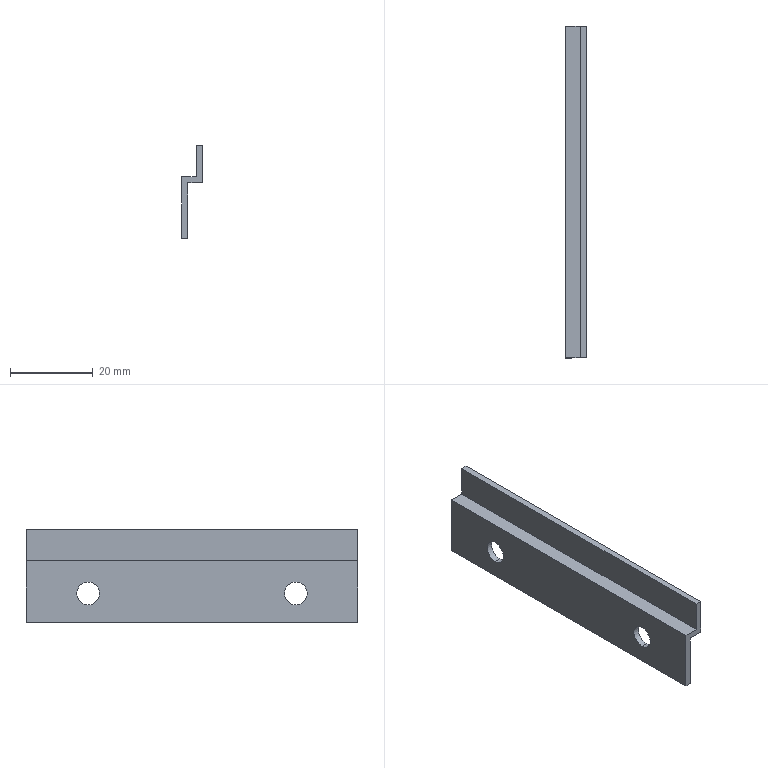Part | SolidWorks | features BaseBody 1 | 1 solid | 14 faces | box 5 x 80 x 22.4 mm | volume 3037 mm3 | plane 10 | cylinder 4 | commonest cylinder face diameters 5.5 x4
STEP:
#1=CARTESIAN_POINT('',(881.946,-4070.973,1937.721));
#2=VERTEX_POINT('',#1);
#3=CARTESIAN_POINT('',(881.946,-4070.973,1932.221));
#4=VERTEX_POINT('',#3);
#5=CARTESIAN_POINT('',(881.946,-4070.973,1934.971));
#6=DIRECTION('',(1.,0.,0.));
#7=DIRECTION('',(0.,0.,-1.));
#8=AXIS2_PLACEMENT_3D('',#5,#6,#7);
#9=CIRCLE('',#8,2.75);
#10=EDGE_CURVE('',#2,#4,#9,.T.);
#11=ORIENTED_EDGE('',*,*,#10,.F.);
#12=CARTESIAN_POINT('',(883.446,-4070.973,1937.721));
#13=VERTEX_POINT('',#12);
#14=CARTESIAN_POINT('',(886.325,-4070.973,1937.721));
#15=DIRECTION('',(1.,0.,0.));
#16=VECTOR('',#15,1000.);
#17=LINE('',#14,#16);
#18=EDGE_CURVE('',#2,#13,#17,.T.);
#19=ORIENTED_EDGE('',*,*,#18,.T.);
#20=CARTESIAN_POINT('',(883.446,-4070.973,1932.221));
#21=VERTEX_POINT('',#20);
#22=CARTESIAN_POINT('',(883.446,-4070.973,1934.971));
#23=DIRECTION('',(-1.,0.,0.));
#24=DIRECTION('',(0.,0.,-1.));
#25=AXIS2_PLACEMENT_3D('',#22,#23,#24);
#26=CIRCLE('',#25,2.75);
#27=EDGE_CURVE('',#21,#13,#26,.T.);
#28=ORIENTED_EDGE('',*,*,#27,.F.);
#29=CARTESIAN_POINT('',(886.325,-4070.973,1932.221));
#30=DIRECTION('',(1.,0.,0.));
#31=VECTOR('',#30,1000.);
#32=LINE('',#29,#31);
#33=EDGE_CURVE('',#4,#21,#32,.T.);
#34=ORIENTED_EDGE('',*,*,#33,.F.);
#35=EDGE_LOOP('',(#11,#19,#28,#34));
#36=FACE_OUTER_BOUND('',#35,.T.);
#37=CARTESIAN_POINT('',(886.325,-4070.973,1934.971));
#38=DIRECTION('',(1.,0.,0.));
#39=DIRECTION('',(0.,0.,-1.));
#40=AXIS2_PLACEMENT_3D('',#37,#38,#39);
#41=CYLINDRICAL_SURFACE('',#40,2.75);
#42=ADVANCED_FACE('',(#36),#41,.F.);
#43=CARTESIAN_POINT('',(883.446,-4020.973,1932.221));
#44=VERTEX_POINT('',#43);
#45=CARTESIAN_POINT('',(883.446,-4020.973,1937.721));
#46=VERTEX_POINT('',#45);
#47=CARTESIAN_POINT('',(883.446,-4020.973,1934.971));
#48=DIRECTION('',(-1.,0.,0.));
#49=DIRECTION('',(0.,0.,1.));
#50=AXIS2_PLACEMENT_3D('',#47,#48,#49);
#51=CIRCLE('',#50,2.75);
#52=EDGE_CURVE('',#44,#46,#51,.T.);
#53=ORIENTED_EDGE('',*,*,#52,.F.);
#54=CARTESIAN_POINT('',(881.946,-4020.973,1932.221));
#55=VERTEX_POINT('',#54);
#56=CARTESIAN_POINT('',(886.325,-4020.973,1932.221));
#57=DIRECTION('',(-1.,0.,0.));
#58=VECTOR('',#57,1000.);
#59=LINE('',#56,#58);
#60=EDGE_CURVE('',#44,#55,#59,.T.);
#61=ORIENTED_EDGE('',*,*,#60,.T.);
#62=CARTESIAN_POINT('',(881.946,-4020.973,1937.721));
#63=VERTEX_POINT('',#62);
#64=CARTESIAN_POINT('',(881.946,-4020.973,1934.971));
#65=DIRECTION('',(1.,0.,0.));
#66=DIRECTION('',(0.,0.,1.));
#67=AXIS2_PLACEMENT_3D('',#64,#65,#66);
#68=CIRCLE('',#67,2.75);
#69=EDGE_CURVE('',#63,#55,#68,.T.);
#70=ORIENTED_EDGE('',*,*,#69,.F.);
#71=CARTESIAN_POINT('',(886.325,-4020.973,1937.721));
#72=DIRECTION('',(-1.,0.,0.));
#73=VECTOR('',#72,1000.);
#74=LINE('',#71,#73);
#75=EDGE_CURVE('',#46,#63,#74,.T.);
#76=ORIENTED_EDGE('',*,*,#75,.F.);
#77=EDGE_LOOP('',(#53,#61,#70,#76));
#78=FACE_OUTER_BOUND('',#77,.T.);
#79=CARTESIAN_POINT('',(886.325,-4020.973,1934.971));
#80=DIRECTION('',(-1.,0.,0.));
#81=DIRECTION('',(0.,0.,1.));
#82=AXIS2_PLACEMENT_3D('',#79,#80,#81);
#83=CYLINDRICAL_SURFACE('',#82,2.75);
#84=ADVANCED_FACE('',(#78),#83,.F.);
#85=CARTESIAN_POINT('',(881.946,-4005.973,1942.871));
#86=VERTEX_POINT('',#85);
#87=CARTESIAN_POINT('',(881.946,-4005.973,1927.971));
#88=VERTEX_POINT('',#87);
#89=CARTESIAN_POINT('',(881.946,-4005.973,1927.971));
#90=DIRECTION('',(0.,0.,-1.));
#91=VECTOR('',#90,1000.);
#92=LINE('',#89,#91);
#93=EDGE_CURVE('',#86,#88,#92,.T.);
#94=ORIENTED_EDGE('',*,*,#93,.T.);
#95=CARTESIAN_POINT('',(881.946,-4085.973,1927.971));
#96=VERTEX_POINT('',#95);
#97=CARTESIAN_POINT('',(881.946,-4005.973,1927.971));
#98=DIRECTION('',(0.,-1.,0.));
#99=VECTOR('',#98,1000.);
#100=LINE('',#97,#99);
#101=EDGE_CURVE('',#88,#96,#100,.T.);
#102=ORIENTED_EDGE('',*,*,#101,.T.);
#103=CARTESIAN_POINT('',(881.946,-4085.973,1942.871));
#104=VERTEX_POINT('',#103);
#105=CARTESIAN_POINT('',(881.946,-4085.973,1927.971));
#106=DIRECTION('',(0.,0.,1.));
#107=VECTOR('',#106,1000.);
#108=LINE('',#105,#107);
#109=EDGE_CURVE('',#96,#104,#108,.T.);
#110=ORIENTED_EDGE('',*,*,#109,.T.);
#111=CARTESIAN_POINT('',(881.946,-4005.973,1942.871));
#112=DIRECTION('',(0.,1.,0.));
#113=VECTOR('',#112,1000.);
#114=LINE('',#111,#113);
#115=EDGE_CURVE('',#104,#86,#114,.T.);
#116=ORIENTED_EDGE('',*,*,#115,.T.);
#117=EDGE_LOOP('',(#94,#102,#110,#116));
#118=FACE_OUTER_BOUND('',#117,.T.);
#119=CARTESIAN_POINT('',(881.946,-4070.973,1934.971));
#120=DIRECTION('',(1.,0.,0.));
#121=DIRECTION('',(0.,0.,-1.));
#122=AXIS2_PLACEMENT_3D('',#119,#120,#121);
#123=CIRCLE('',#122,2.75);
#124=EDGE_CURVE('',#4,#2,#123,.T.);
#125=ORIENTED_EDGE('',*,*,#124,.T.);
#126=ORIENTED_EDGE('',*,*,#10,.T.);
#127=EDGE_LOOP('',(#125,#126));
#128=FACE_BOUND('',#127,.T.);
#129=ORIENTED_EDGE('',*,*,#69,.T.);
#130=CARTESIAN_POINT('',(881.946,-4020.973,1934.971));
#131=DIRECTION('',(1.,0.,0.));
#132=DIRECTION('',(0.,0.,1.));
#133=AXIS2_PLACEMENT_3D('',#130,#131,#132);
#134=CIRCLE('',#133,2.75);
#135=EDGE_CURVE('',#55,#63,#134,.T.);
#136=ORIENTED_EDGE('',*,*,#135,.T.);
#137=EDGE_LOOP('',(#129,#136));
#138=FACE_BOUND('',#137,.T.);
#139=CARTESIAN_POINT('',(881.946,-4005.973,1927.971));
#140=DIRECTION('',(-1.,0.,0.));
#141=DIRECTION('',(0.,0.,1.));
#142=AXIS2_PLACEMENT_3D('',#139,#140,#141);
#143=PLANE('',#142);
#144=ADVANCED_FACE('',(#118,#128,#138),#143,.T.);
#145=CARTESIAN_POINT('',(883.446,-4005.973,1927.971));
#146=VERTEX_POINT('',#145);
#147=CARTESIAN_POINT('',(883.446,-4005.973,1927.971));
#148=DIRECTION('',(1.,0.,0.));
#149=VECTOR('',#148,1000.);
#150=LINE('',#147,#149);
#151=EDGE_CURVE('',#88,#146,#150,.T.);
#152=ORIENTED_EDGE('',*,*,#151,.T.);
#153=CARTESIAN_POINT('',(883.446,-4085.973,1927.971));
#154=VERTEX_POINT('',#153);
#155=CARTESIAN_POINT('',(883.446,-4005.973,1927.971));
#156=DIRECTION('',(0.,-1.,0.));
#157=VECTOR('',#156,1000.);
#158=LINE('',#155,#157);
#159=EDGE_CURVE('',#146,#154,#158,.T.);
#160=ORIENTED_EDGE('',*,*,#159,.T.);
#161=CARTESIAN_POINT('',(883.446,-4085.973,1927.971));
#162=DIRECTION('',(-1.,0.,0.));
#163=VECTOR('',#162,1000.);
#164=LINE('',#161,#163);
#165=EDGE_CURVE('',#154,#96,#164,.T.);
#166=ORIENTED_EDGE('',*,*,#165,.T.);
#167=ORIENTED_EDGE('',*,*,#101,.F.);
#168=EDGE_LOOP('',(#152,#160,#166,#167));
#169=FACE_OUTER_BOUND('',#168,.T.);
#170=CARTESIAN_POINT('',(883.446,-4005.973,1927.971));
#171=DIRECTION('',(0.,0.,-1.));
#172=DIRECTION('',(-1.,0.,0.));
#173=AXIS2_PLACEMENT_3D('',#170,#171,#172);
#174=PLANE('',#173);
#175=ADVANCED_FACE('',(#169),#174,.T.);
#176=CARTESIAN_POINT('',(885.446,-4005.973,1942.871));
#177=VERTEX_POINT('',#176);
#178=CARTESIAN_POINT('',(885.446,-4005.973,1950.371));
#179=VERTEX_POINT('',#178);
#180=CARTESIAN_POINT('',(885.446,-4005.973,1939.548));
#181=DIRECTION('',(0.,0.,1.));
#182=VECTOR('',#181,1000.);
#183=LINE('',#180,#182);
#184=EDGE_CURVE('',#177,#179,#183,.T.);
#185=ORIENTED_EDGE('',*,*,#184,.T.);
#186=CARTESIAN_POINT('',(886.946,-4005.973,1950.371));
#187=VERTEX_POINT('',#186);
#188=CARTESIAN_POINT('',(885.446,-4005.973,1950.371));
#189=DIRECTION('',(-1.,0.,0.));
#190=VECTOR('',#189,1000.);
#191=LINE('',#188,#190);
#192=EDGE_CURVE('',#187,#179,#191,.T.);
#193=ORIENTED_EDGE('',*,*,#192,.F.);
#194=CARTESIAN_POINT('',(886.946,-4005.973,1941.371));
#195=VERTEX_POINT('',#194);
#196=CARTESIAN_POINT('',(886.946,-4005.973,1939.548));
#197=DIRECTION('',(0.,0.,-1.));
#198=VECTOR('',#197,1000.);
#199=LINE('',#196,#198);
#200=EDGE_CURVE('',#187,#195,#199,.T.);
#201=ORIENTED_EDGE('',*,*,#200,.T.);
#202=CARTESIAN_POINT('',(883.446,-4005.973,1941.371));
#203=VERTEX_POINT('',#202);
#204=CARTESIAN_POINT('',(884.069,-4005.973,1941.371));
#205=DIRECTION('',(-1.,0.,0.));
#206=VECTOR('',#205,1000.);
#207=LINE('',#204,#206);
#208=EDGE_CURVE('',#195,#203,#207,.T.);
#209=ORIENTED_EDGE('',*,*,#208,.T.);
#210=CARTESIAN_POINT('',(883.446,-4005.973,1939.548));
#211=DIRECTION('',(0.,0.,-1.));
#212=VECTOR('',#211,1000.);
#213=LINE('',#210,#212);
#214=EDGE_CURVE('',#203,#146,#213,.T.);
#215=ORIENTED_EDGE('',*,*,#214,.T.);
#216=ORIENTED_EDGE('',*,*,#151,.F.);
#217=ORIENTED_EDGE('',*,*,#93,.F.);
#218=CARTESIAN_POINT('',(884.069,-4005.973,1942.871));
#219=DIRECTION('',(1.,0.,0.));
#220=VECTOR('',#219,1000.);
#221=LINE('',#218,#220);
#222=EDGE_CURVE('',#86,#177,#221,.T.);
#223=ORIENTED_EDGE('',*,*,#222,.T.);
#224=EDGE_LOOP('',(#185,#193,#201,#209,#215,#216,#217,#223));
#225=FACE_OUTER_BOUND('',#224,.T.);
#226=CARTESIAN_POINT('',(884.069,-4005.973,1939.548));
#227=DIRECTION('',(0.,1.,0.));
#228=DIRECTION('',(0.,0.,1.));
#229=AXIS2_PLACEMENT_3D('',#226,#227,#228);
#230=PLANE('',#229);
#231=ADVANCED_FACE('',(#225),#230,.T.);
#232=ORIENTED_EDGE('',*,*,#222,.F.);
#233=ORIENTED_EDGE('',*,*,#115,.F.);
#234=CARTESIAN_POINT('',(885.446,-4085.973,1942.871));
#235=VERTEX_POINT('',#234);
#236=CARTESIAN_POINT('',(881.946,-4085.973,1942.871));
#237=DIRECTION('',(1.,0.,0.));
#238=VECTOR('',#237,1000.);
#239=LINE('',#236,#238);
#240=EDGE_CURVE('',#104,#235,#239,.T.);
#241=ORIENTED_EDGE('',*,*,#240,.T.);
#242=CARTESIAN_POINT('',(885.446,-4005.973,1942.871));
#243=DIRECTION('',(0.,1.,0.));
#244=VECTOR('',#243,1000.);
#245=LINE('',#242,#244);
#246=EDGE_CURVE('',#235,#177,#245,.T.);
#247=ORIENTED_EDGE('',*,*,#246,.T.);
#248=EDGE_LOOP('',(#232,#233,#241,#247));
#249=FACE_OUTER_BOUND('',#248,.T.);
#250=CARTESIAN_POINT('',(881.946,-4005.973,1942.871));
#251=DIRECTION('',(0.,0.,1.));
#252=DIRECTION('',(1.,0.,0.));
#253=AXIS2_PLACEMENT_3D('',#250,#251,#252);
#254=PLANE('',#253);
#255=ADVANCED_FACE('',(#249),#254,.T.);
#256=CARTESIAN_POINT('',(886.946,-4085.973,1950.371));
#257=VERTEX_POINT('',#256);
#258=CARTESIAN_POINT('',(886.946,-4085.973,1941.371));
#259=VERTEX_POINT('',#258);
#260=CARTESIAN_POINT('',(886.946,-4085.973,1939.548));
#261=DIRECTION('',(0.,0.,-1.));
#262=VECTOR('',#261,1000.);
#263=LINE('',#260,#262);
#264=EDGE_CURVE('',#257,#259,#263,.T.);
#265=ORIENTED_EDGE('',*,*,#264,.F.);
#266=CARTESIAN_POINT('',(885.446,-4085.973,1950.371));
#267=VERTEX_POINT('',#266);
#268=CARTESIAN_POINT('',(885.446,-4085.973,1950.371));
#269=DIRECTION('',(1.,0.,0.));
#270=VECTOR('',#269,1000.);
#271=LINE('',#268,#270);
#272=EDGE_CURVE('',#267,#257,#271,.T.);
#273=ORIENTED_EDGE('',*,*,#272,.F.);
#274=CARTESIAN_POINT('',(885.446,-4085.973,1939.548));
#275=DIRECTION('',(0.,0.,1.));
#276=VECTOR('',#275,1000.);
#277=LINE('',#274,#276);
#278=EDGE_CURVE('',#235,#267,#277,.T.);
#279=ORIENTED_EDGE('',*,*,#278,.F.);
#280=ORIENTED_EDGE('',*,*,#240,.F.);
#281=ORIENTED_EDGE('',*,*,#109,.F.);
#282=ORIENTED_EDGE('',*,*,#165,.F.);
#283=CARTESIAN_POINT('',(883.446,-4085.973,1941.371));
#284=VERTEX_POINT('',#283);
#285=CARTESIAN_POINT('',(883.446,-4085.973,1939.548));
#286=DIRECTION('',(0.,0.,-1.));
#287=VECTOR('',#286,1000.);
#288=LINE('',#285,#287);
#289=EDGE_CURVE('',#284,#154,#288,.T.);
#290=ORIENTED_EDGE('',*,*,#289,.F.);
#291=CARTESIAN_POINT('',(884.069,-4085.973,1941.371));
#292=DIRECTION('',(-1.,0.,0.));
#293=VECTOR('',#292,1000.);
#294=LINE('',#291,#293);
#295=EDGE_CURVE('',#259,#284,#294,.T.);
#296=ORIENTED_EDGE('',*,*,#295,.F.);
#297=EDGE_LOOP('',(#265,#273,#279,#280,#281,#282,#290,#296));
#298=FACE_OUTER_BOUND('',#297,.T.);
#299=CARTESIAN_POINT('',(884.069,-4085.973,1939.548));
#300=DIRECTION('',(0.,1.,0.));
#301=DIRECTION('',(0.,0.,1.));
#302=AXIS2_PLACEMENT_3D('',#299,#300,#301);
#303=PLANE('',#302);
#304=ADVANCED_FACE('',(#298),#303,.F.);
#305=ORIENTED_EDGE('',*,*,#18,.F.);
#306=ORIENTED_EDGE('',*,*,#124,.F.);
#307=ORIENTED_EDGE('',*,*,#33,.T.);
#308=CARTESIAN_POINT('',(883.446,-4070.973,1934.971));
#309=DIRECTION('',(-1.,0.,0.));
#310=DIRECTION('',(0.,0.,-1.));
#311=AXIS2_PLACEMENT_3D('',#308,#309,#310);
#312=CIRCLE('',#311,2.75);
#313=EDGE_CURVE('',#13,#21,#312,.T.);
#314=ORIENTED_EDGE('',*,*,#313,.F.);
#315=EDGE_LOOP('',(#305,#306,#307,#314));
#316=FACE_OUTER_BOUND('',#315,.T.);
#317=CARTESIAN_POINT('',(886.325,-4070.973,1934.971));
#318=DIRECTION('',(1.,0.,0.));
#319=DIRECTION('',(0.,0.,-1.));
#320=AXIS2_PLACEMENT_3D('',#317,#318,#319);
#321=CYLINDRICAL_SURFACE('',#320,2.75);
#322=ADVANCED_FACE('',(#316),#321,.F.);
#323=ORIENTED_EDGE('',*,*,#60,.F.);
#324=CARTESIAN_POINT('',(883.446,-4020.973,1934.971));
#325=DIRECTION('',(-1.,0.,0.));
#326=DIRECTION('',(0.,0.,1.));
#327=AXIS2_PLACEMENT_3D('',#324,#325,#326);
#328=CIRCLE('',#327,2.75);
#329=EDGE_CURVE('',#46,#44,#328,.T.);
#330=ORIENTED_EDGE('',*,*,#329,.F.);
#331=ORIENTED_EDGE('',*,*,#75,.T.);
#332=ORIENTED_EDGE('',*,*,#135,.F.);
#333=EDGE_LOOP('',(#323,#330,#331,#332));
#334=FACE_OUTER_BOUND('',#333,.T.);
#335=CARTESIAN_POINT('',(886.325,-4020.973,1934.971));
#336=DIRECTION('',(-1.,0.,0.));
#337=DIRECTION('',(0.,0.,1.));
#338=AXIS2_PLACEMENT_3D('',#335,#336,#337);
#339=CYLINDRICAL_SURFACE('',#338,2.75);
#340=ADVANCED_FACE('',(#334),#339,.F.);
#341=ORIENTED_EDGE('',*,*,#214,.F.);
#342=CARTESIAN_POINT('',(883.446,-4005.973,1941.371));
#343=DIRECTION('',(0.,-1.,0.));
#344=VECTOR('',#343,1000.);
#345=LINE('',#342,#344);
#346=EDGE_CURVE('',#203,#284,#345,.T.);
#347=ORIENTED_EDGE('',*,*,#346,.T.);
#348=ORIENTED_EDGE('',*,*,#289,.T.);
#349=ORIENTED_EDGE('',*,*,#159,.F.);
#350=EDGE_LOOP('',(#341,#347,#348,#349));
#351=FACE_OUTER_BOUND('',#350,.T.);
#352=ORIENTED_EDGE('',*,*,#27,.T.);
#353=ORIENTED_EDGE('',*,*,#313,.T.);
#354=EDGE_LOOP('',(#352,#353));
#355=FACE_BOUND('',#354,.T.);
#356=ORIENTED_EDGE('',*,*,#329,.T.);
#357=ORIENTED_EDGE('',*,*,#52,.T.);
#358=EDGE_LOOP('',(#356,#357));
#359=FACE_BOUND('',#358,.T.);
#360=CARTESIAN_POINT('',(883.446,-4005.973,1941.371));
#361=DIRECTION('',(1.,0.,0.));
#362=DIRECTION('',(0.,0.,-1.));
#363=AXIS2_PLACEMENT_3D('',#360,#361,#362);
#364=PLANE('',#363);
#365=ADVANCED_FACE('',(#351,#355,#359),#364,.T.);
#366=ORIENTED_EDGE('',*,*,#184,.F.);
#367=ORIENTED_EDGE('',*,*,#246,.F.);
#368=ORIENTED_EDGE('',*,*,#278,.T.);
#369=CARTESIAN_POINT('',(885.446,-4005.973,1950.371));
#370=DIRECTION('',(0.,1.,0.));
#371=VECTOR('',#370,1000.);
#372=LINE('',#369,#371);
#373=EDGE_CURVE('',#267,#179,#372,.T.);
#374=ORIENTED_EDGE('',*,*,#373,.T.);
#375=EDGE_LOOP('',(#366,#367,#368,#374));
#376=FACE_OUTER_BOUND('',#375,.T.);
#377=CARTESIAN_POINT('',(885.446,-4005.973,1942.871));
#378=DIRECTION('',(-1.,0.,0.));
#379=DIRECTION('',(0.,0.,1.));
#380=AXIS2_PLACEMENT_3D('',#377,#378,#379);
#381=PLANE('',#380);
#382=ADVANCED_FACE('',(#376),#381,.T.);
#383=ORIENTED_EDGE('',*,*,#208,.F.);
#384=CARTESIAN_POINT('',(886.946,-4005.973,1941.371));
#385=DIRECTION('',(0.,-1.,0.));
#386=VECTOR('',#385,1000.);
#387=LINE('',#384,#386);
#388=EDGE_CURVE('',#195,#259,#387,.T.);
#389=ORIENTED_EDGE('',*,*,#388,.T.);
#390=ORIENTED_EDGE('',*,*,#295,.T.);
#391=ORIENTED_EDGE('',*,*,#346,.F.);
#392=EDGE_LOOP('',(#383,#389,#390,#391));
#393=FACE_OUTER_BOUND('',#392,.T.);
#394=CARTESIAN_POINT('',(886.946,-4005.973,1941.371));
#395=DIRECTION('',(0.,0.,-1.));
#396=DIRECTION('',(-1.,0.,0.));
#397=AXIS2_PLACEMENT_3D('',#394,#395,#396);
#398=PLANE('',#397);
#399=ADVANCED_FACE('',(#393),#398,.T.);
#400=ORIENTED_EDGE('',*,*,#200,.F.);
#401=CARTESIAN_POINT('',(886.946,-4005.973,1950.371));
#402=DIRECTION('',(0.,-1.,0.));
#403=VECTOR('',#402,1000.);
#404=LINE('',#401,#403);
#405=EDGE_CURVE('',#187,#257,#404,.T.);
#406=ORIENTED_EDGE('',*,*,#405,.T.);
#407=ORIENTED_EDGE('',*,*,#264,.T.);
#408=ORIENTED_EDGE('',*,*,#388,.F.);
#409=EDGE_LOOP('',(#400,#406,#407,#408));
#410=FACE_OUTER_BOUND('',#409,.T.);
#411=CARTESIAN_POINT('',(886.946,-4005.973,1950.371));
#412=DIRECTION('',(1.,0.,0.));
#413=DIRECTION('',(0.,0.,-1.));
#414=AXIS2_PLACEMENT_3D('',#411,#412,#413);
#415=PLANE('',#414);
#416=ADVANCED_FACE('',(#410),#415,.T.);
#417=ORIENTED_EDGE('',*,*,#192,.T.);
#418=ORIENTED_EDGE('',*,*,#373,.F.);
#419=ORIENTED_EDGE('',*,*,#272,.T.);
#420=ORIENTED_EDGE('',*,*,#405,.F.);
#421=EDGE_LOOP('',(#417,#418,#419,#420));
#422=FACE_OUTER_BOUND('',#421,.T.);
#423=CARTESIAN_POINT('',(885.446,-4005.973,1950.371));
#424=DIRECTION('',(0.,0.,1.));
#425=DIRECTION('',(1.,0.,0.));
#426=AXIS2_PLACEMENT_3D('',#423,#424,#425);
#427=PLANE('',#426);
#428=ADVANCED_FACE('',(#422),#427,.T.);
#429=CLOSED_SHELL('',(#42,#84,#144,#175,#231,#255,#304,#322,#340,#365,#382,#399,#416,#428));
#430=MANIFOLD_SOLID_BREP('',#429);
#431=CARTESIAN_POINT('',(0.,0.,0.));
#432=DIRECTION('',(0.,0.,1.));
#433=DIRECTION('',(1.,0.,0.));
#434=AXIS2_PLACEMENT_3D('',#431,#432,#433);
#435=(LENGTH_UNIT()NAMED_UNIT(*)SI_UNIT(.MILLI.,.METRE.));
#436=UNCERTAINTY_MEASURE_WITH_UNIT(LENGTH_MEASURE(0.00001),#435,'','');
#437=(NAMED_UNIT(*)PLANE_ANGLE_UNIT()SI_UNIT($,.RADIAN.));
#438=(NAMED_UNIT(*)SI_UNIT($,.STERADIAN.)SOLID_ANGLE_UNIT());
#439=(GEOMETRIC_REPRESENTATION_CONTEXT(3)GLOBAL_UNCERTAINTY_ASSIGNED_CONTEXT((#436))GLOBAL_UNIT_ASSIGNED_CONTEXT((#435,#437,#438))REPRESENTATION_CONTEXT('',''));
#440=ADVANCED_BREP_SHAPE_REPRESENTATION('',(#430,#434),#439);